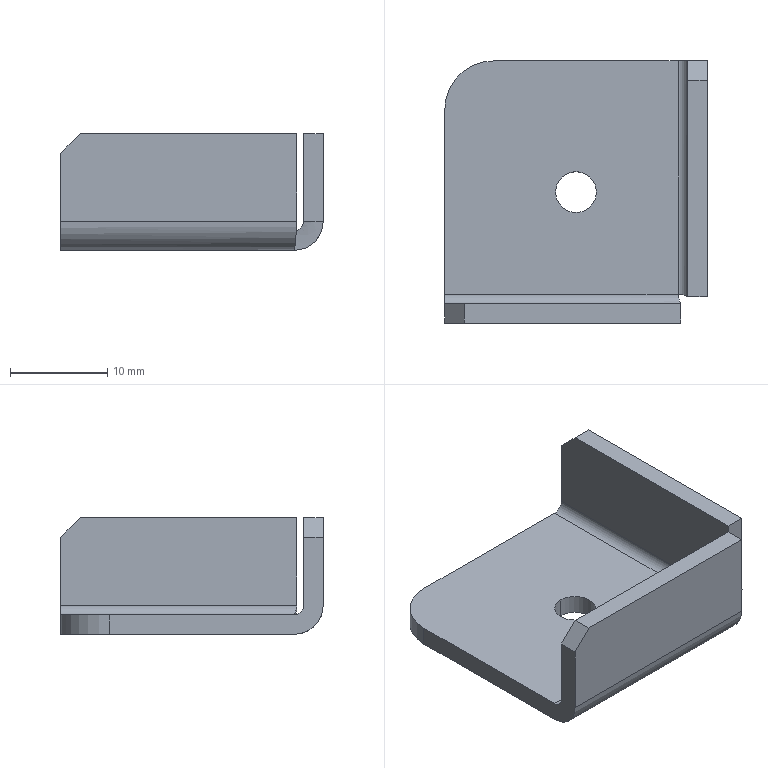Part | STEP file | OP02-QR01-J618 | 1 solid | 23 faces | box 27 x 27 x 12 mm | volume 2284 mm3 | plane 14 | cylinder 7 | spline 2 | commonest cylinder face diameters 2 x2 4.2 x2 6 x2 10 x1